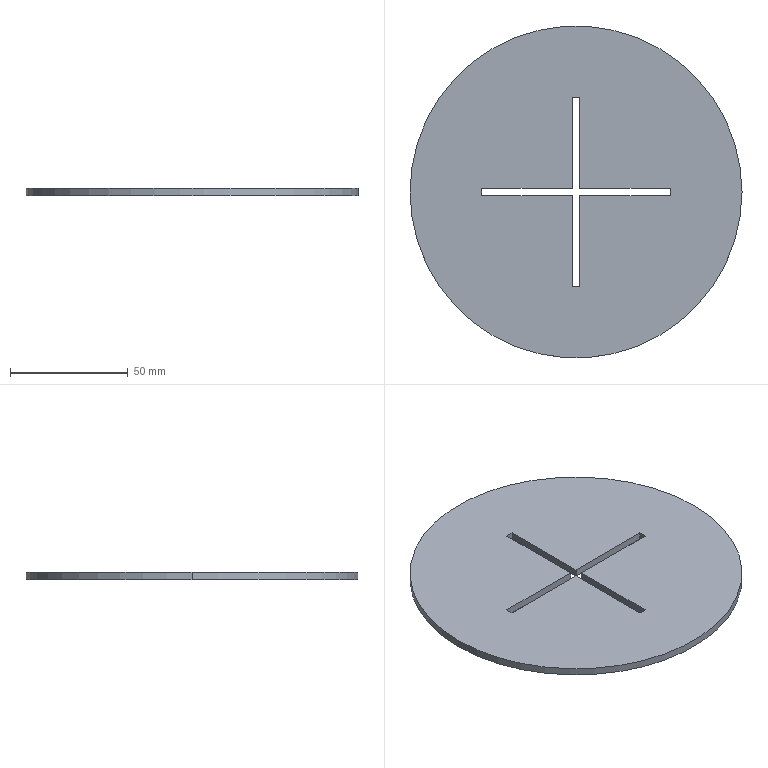Part | SolidWorks | features FlatPattern 1, SMBaseFlange 1, SheetMetal 1 | 1 solid | 16 faces | box 141 x 141 x 3.2 mm | volume 48361 mm3 | plane 14 | cylinder 2 | commonest cylinder face diameters 141 x2
STEP:
#1=CARTESIAN_POINT('',(46.57,-1.6,3.2));
#2=VERTEX_POINT('',#1);
#3=CARTESIAN_POINT('',(-94.43,-1.6,3.2));
#4=VERTEX_POINT('',#3);
#5=CARTESIAN_POINT('',(-23.93,-1.6,3.2));
#6=DIRECTION('',(0.,0.,1.));
#7=DIRECTION('',(1.,0.,0.));
#8=AXIS2_PLACEMENT_3D('',#5,#6,#7);
#9=CIRCLE('',#8,70.5);
#10=EDGE_CURVE('',#2,#4,#9,.T.);
#11=ORIENTED_EDGE('',*,*,#10,.F.);
#12=CARTESIAN_POINT('',(46.57,-1.6,0.));
#13=VERTEX_POINT('',#12);
#14=CARTESIAN_POINT('',(46.57,-1.6,3.2));
#15=DIRECTION('',(0.,0.,-1.));
#16=VECTOR('',#15,1000.);
#17=LINE('',#14,#16);
#18=EDGE_CURVE('',#2,#13,#17,.T.);
#19=ORIENTED_EDGE('',*,*,#18,.T.);
#20=CARTESIAN_POINT('',(-94.43,-1.6,0.));
#21=VERTEX_POINT('',#20);
#22=CARTESIAN_POINT('',(-23.93,-1.6,0.));
#23=DIRECTION('',(0.,0.,1.));
#24=DIRECTION('',(1.,0.,0.));
#25=AXIS2_PLACEMENT_3D('',#22,#23,#24);
#26=CIRCLE('',#25,70.5);
#27=EDGE_CURVE('',#13,#21,#26,.T.);
#28=ORIENTED_EDGE('',*,*,#27,.T.);
#29=CARTESIAN_POINT('',(-94.43,-1.6,3.2));
#30=DIRECTION('',(0.,0.,-1.));
#31=VECTOR('',#30,1000.);
#32=LINE('',#29,#31);
#33=EDGE_CURVE('',#4,#21,#32,.T.);
#34=ORIENTED_EDGE('',*,*,#33,.F.);
#35=EDGE_LOOP('',(#11,#19,#28,#34));
#36=FACE_OUTER_BOUND('',#35,.T.);
#37=CARTESIAN_POINT('',(-23.93,-1.6,3.2));
#38=DIRECTION('',(0.,0.,-1.));
#39=DIRECTION('',(-1.,0.,0.));
#40=AXIS2_PLACEMENT_3D('',#37,#38,#39);
#41=CYLINDRICAL_SURFACE('',#40,70.5);
#42=ADVANCED_FACE('',(#36),#41,.T.);
#43=CARTESIAN_POINT('',(-23.93,-1.6,3.2));
#44=DIRECTION('',(0.,0.,1.));
#45=DIRECTION('',(1.,0.,0.));
#46=AXIS2_PLACEMENT_3D('',#43,#44,#45);
#47=CIRCLE('',#46,70.5);
#48=EDGE_CURVE('',#4,#2,#47,.T.);
#49=ORIENTED_EDGE('',*,*,#48,.T.);
#50=ORIENTED_EDGE('',*,*,#10,.T.);
#51=EDGE_LOOP('',(#49,#50));
#52=FACE_OUTER_BOUND('',#51,.T.);
#53=CARTESIAN_POINT('',(-63.93,-3.2,3.2));
#54=VERTEX_POINT('',#53);
#55=CARTESIAN_POINT('',(-25.53,-3.2,3.2));
#56=VERTEX_POINT('',#55);
#57=CARTESIAN_POINT('',(-63.93,-3.2,3.2));
#58=DIRECTION('',(1.,0.,0.));
#59=VECTOR('',#58,1000.);
#60=LINE('',#57,#59);
#61=EDGE_CURVE('',#54,#56,#60,.T.);
#62=ORIENTED_EDGE('',*,*,#61,.F.);
#63=CARTESIAN_POINT('',(-63.93,0.,3.2));
#64=VERTEX_POINT('',#63);
#65=CARTESIAN_POINT('',(-63.93,0.,3.2));
#66=DIRECTION('',(0.,-1.,0.));
#67=VECTOR('',#66,1000.);
#68=LINE('',#65,#67);
#69=EDGE_CURVE('',#64,#54,#68,.T.);
#70=ORIENTED_EDGE('',*,*,#69,.F.);
#71=CARTESIAN_POINT('',(-25.53,0.,3.2));
#72=VERTEX_POINT('',#71);
#73=CARTESIAN_POINT('',(-25.53,0.,3.2));
#74=DIRECTION('',(-1.,0.,0.));
#75=VECTOR('',#74,1000.);
#76=LINE('',#73,#75);
#77=EDGE_CURVE('',#72,#64,#76,.T.);
#78=ORIENTED_EDGE('',*,*,#77,.F.);
#79=CARTESIAN_POINT('',(-25.53,38.4,3.2));
#80=VERTEX_POINT('',#79);
#81=CARTESIAN_POINT('',(-25.53,38.4,3.2));
#82=DIRECTION('',(0.,-1.,0.));
#83=VECTOR('',#82,1000.);
#84=LINE('',#81,#83);
#85=EDGE_CURVE('',#80,#72,#84,.T.);
#86=ORIENTED_EDGE('',*,*,#85,.F.);
#87=CARTESIAN_POINT('',(-22.33,38.4,3.2));
#88=VERTEX_POINT('',#87);
#89=CARTESIAN_POINT('',(-25.53,38.4,3.2));
#90=DIRECTION('',(-1.,0.,0.));
#91=VECTOR('',#90,1000.);
#92=LINE('',#89,#91);
#93=EDGE_CURVE('',#88,#80,#92,.T.);
#94=ORIENTED_EDGE('',*,*,#93,.F.);
#95=CARTESIAN_POINT('',(-22.33,0.,3.2));
#96=VERTEX_POINT('',#95);
#97=CARTESIAN_POINT('',(-22.33,38.4,3.2));
#98=DIRECTION('',(0.,1.,0.));
#99=VECTOR('',#98,1000.);
#100=LINE('',#97,#99);
#101=EDGE_CURVE('',#96,#88,#100,.T.);
#102=ORIENTED_EDGE('',*,*,#101,.F.);
#103=CARTESIAN_POINT('',(16.07,0.,3.2));
#104=VERTEX_POINT('',#103);
#105=CARTESIAN_POINT('',(16.07,0.,3.2));
#106=DIRECTION('',(-1.,0.,0.));
#107=VECTOR('',#106,1000.);
#108=LINE('',#105,#107);
#109=EDGE_CURVE('',#104,#96,#108,.T.);
#110=ORIENTED_EDGE('',*,*,#109,.F.);
#111=CARTESIAN_POINT('',(16.07,-3.2,3.2));
#112=VERTEX_POINT('',#111);
#113=CARTESIAN_POINT('',(16.07,-3.2,3.2));
#114=DIRECTION('',(0.,1.,0.));
#115=VECTOR('',#114,1000.);
#116=LINE('',#113,#115);
#117=EDGE_CURVE('',#112,#104,#116,.T.);
#118=ORIENTED_EDGE('',*,*,#117,.F.);
#119=CARTESIAN_POINT('',(-22.33,-3.2,3.2));
#120=VERTEX_POINT('',#119);
#121=CARTESIAN_POINT('',(-22.33,-3.2,3.2));
#122=DIRECTION('',(1.,0.,0.));
#123=VECTOR('',#122,1000.);
#124=LINE('',#121,#123);
#125=EDGE_CURVE('',#120,#112,#124,.T.);
#126=ORIENTED_EDGE('',*,*,#125,.F.);
#127=CARTESIAN_POINT('',(-22.33,-41.6,3.2));
#128=VERTEX_POINT('',#127);
#129=CARTESIAN_POINT('',(-22.33,-3.2,3.2));
#130=DIRECTION('',(0.,1.,0.));
#131=VECTOR('',#130,1000.);
#132=LINE('',#129,#131);
#133=EDGE_CURVE('',#128,#120,#132,.T.);
#134=ORIENTED_EDGE('',*,*,#133,.F.);
#135=CARTESIAN_POINT('',(-25.53,-41.6,3.2));
#136=VERTEX_POINT('',#135);
#137=CARTESIAN_POINT('',(-25.53,-41.6,3.2));
#138=DIRECTION('',(1.,0.,0.));
#139=VECTOR('',#138,1000.);
#140=LINE('',#137,#139);
#141=EDGE_CURVE('',#136,#128,#140,.T.);
#142=ORIENTED_EDGE('',*,*,#141,.F.);
#143=CARTESIAN_POINT('',(-25.53,-3.2,3.2));
#144=DIRECTION('',(0.,-1.,0.));
#145=VECTOR('',#144,1000.);
#146=LINE('',#143,#145);
#147=EDGE_CURVE('',#56,#136,#146,.T.);
#148=ORIENTED_EDGE('',*,*,#147,.F.);
#149=EDGE_LOOP('',(#62,#70,#78,#86,#94,#102,#110,#118,#126,#134,#142,#148));
#150=FACE_BOUND('',#149,.T.);
#151=CARTESIAN_POINT('',(-23.93,-1.6,3.2));
#152=DIRECTION('',(0.,0.,1.));
#153=DIRECTION('',(1.,0.,0.));
#154=AXIS2_PLACEMENT_3D('',#151,#152,#153);
#155=PLANE('',#154);
#156=ADVANCED_FACE('',(#52,#150),#155,.T.);
#157=CARTESIAN_POINT('',(-23.93,-1.6,0.));
#158=DIRECTION('',(0.,0.,1.));
#159=DIRECTION('',(1.,0.,0.));
#160=AXIS2_PLACEMENT_3D('',#157,#158,#159);
#161=CIRCLE('',#160,70.5);
#162=EDGE_CURVE('',#21,#13,#161,.T.);
#163=ORIENTED_EDGE('',*,*,#162,.F.);
#164=ORIENTED_EDGE('',*,*,#27,.F.);
#165=EDGE_LOOP('',(#163,#164));
#166=FACE_OUTER_BOUND('',#165,.T.);
#167=CARTESIAN_POINT('',(-63.93,0.,0.));
#168=VERTEX_POINT('',#167);
#169=CARTESIAN_POINT('',(-63.93,-3.2,0.));
#170=VERTEX_POINT('',#169);
#171=CARTESIAN_POINT('',(-63.93,0.,0.));
#172=DIRECTION('',(0.,-1.,0.));
#173=VECTOR('',#172,1000.);
#174=LINE('',#171,#173);
#175=EDGE_CURVE('',#168,#170,#174,.T.);
#176=ORIENTED_EDGE('',*,*,#175,.T.);
#177=CARTESIAN_POINT('',(-25.53,-3.2,0.));
#178=VERTEX_POINT('',#177);
#179=CARTESIAN_POINT('',(-63.93,-3.2,0.));
#180=DIRECTION('',(1.,0.,0.));
#181=VECTOR('',#180,1000.);
#182=LINE('',#179,#181);
#183=EDGE_CURVE('',#170,#178,#182,.T.);
#184=ORIENTED_EDGE('',*,*,#183,.T.);
#185=CARTESIAN_POINT('',(-25.53,-41.6,0.));
#186=VERTEX_POINT('',#185);
#187=CARTESIAN_POINT('',(-25.53,-3.2,0.));
#188=DIRECTION('',(0.,-1.,0.));
#189=VECTOR('',#188,1000.);
#190=LINE('',#187,#189);
#191=EDGE_CURVE('',#178,#186,#190,.T.);
#192=ORIENTED_EDGE('',*,*,#191,.T.);
#193=CARTESIAN_POINT('',(-22.33,-41.6,0.));
#194=VERTEX_POINT('',#193);
#195=CARTESIAN_POINT('',(-25.53,-41.6,0.));
#196=DIRECTION('',(1.,0.,0.));
#197=VECTOR('',#196,1000.);
#198=LINE('',#195,#197);
#199=EDGE_CURVE('',#186,#194,#198,.T.);
#200=ORIENTED_EDGE('',*,*,#199,.T.);
#201=CARTESIAN_POINT('',(-22.33,-3.2,0.));
#202=VERTEX_POINT('',#201);
#203=CARTESIAN_POINT('',(-22.33,-3.2,0.));
#204=DIRECTION('',(0.,1.,0.));
#205=VECTOR('',#204,1000.);
#206=LINE('',#203,#205);
#207=EDGE_CURVE('',#194,#202,#206,.T.);
#208=ORIENTED_EDGE('',*,*,#207,.T.);
#209=CARTESIAN_POINT('',(16.07,-3.2,0.));
#210=VERTEX_POINT('',#209);
#211=CARTESIAN_POINT('',(-22.33,-3.2,0.));
#212=DIRECTION('',(1.,0.,0.));
#213=VECTOR('',#212,1000.);
#214=LINE('',#211,#213);
#215=EDGE_CURVE('',#202,#210,#214,.T.);
#216=ORIENTED_EDGE('',*,*,#215,.T.);
#217=CARTESIAN_POINT('',(16.07,0.,0.));
#218=VERTEX_POINT('',#217);
#219=CARTESIAN_POINT('',(16.07,-3.2,0.));
#220=DIRECTION('',(0.,1.,0.));
#221=VECTOR('',#220,1000.);
#222=LINE('',#219,#221);
#223=EDGE_CURVE('',#210,#218,#222,.T.);
#224=ORIENTED_EDGE('',*,*,#223,.T.);
#225=CARTESIAN_POINT('',(-22.33,0.,0.));
#226=VERTEX_POINT('',#225);
#227=CARTESIAN_POINT('',(16.07,0.,0.));
#228=DIRECTION('',(-1.,0.,0.));
#229=VECTOR('',#228,1000.);
#230=LINE('',#227,#229);
#231=EDGE_CURVE('',#218,#226,#230,.T.);
#232=ORIENTED_EDGE('',*,*,#231,.T.);
#233=CARTESIAN_POINT('',(-22.33,38.4,0.));
#234=VERTEX_POINT('',#233);
#235=CARTESIAN_POINT('',(-22.33,38.4,0.));
#236=DIRECTION('',(0.,1.,0.));
#237=VECTOR('',#236,1000.);
#238=LINE('',#235,#237);
#239=EDGE_CURVE('',#226,#234,#238,.T.);
#240=ORIENTED_EDGE('',*,*,#239,.T.);
#241=CARTESIAN_POINT('',(-25.53,38.4,0.));
#242=VERTEX_POINT('',#241);
#243=CARTESIAN_POINT('',(-25.53,38.4,0.));
#244=DIRECTION('',(-1.,0.,0.));
#245=VECTOR('',#244,1000.);
#246=LINE('',#243,#245);
#247=EDGE_CURVE('',#234,#242,#246,.T.);
#248=ORIENTED_EDGE('',*,*,#247,.T.);
#249=CARTESIAN_POINT('',(-25.53,0.,0.));
#250=VERTEX_POINT('',#249);
#251=CARTESIAN_POINT('',(-25.53,38.4,0.));
#252=DIRECTION('',(0.,-1.,0.));
#253=VECTOR('',#252,1000.);
#254=LINE('',#251,#253);
#255=EDGE_CURVE('',#242,#250,#254,.T.);
#256=ORIENTED_EDGE('',*,*,#255,.T.);
#257=CARTESIAN_POINT('',(-25.53,0.,0.));
#258=DIRECTION('',(-1.,0.,0.));
#259=VECTOR('',#258,1000.);
#260=LINE('',#257,#259);
#261=EDGE_CURVE('',#250,#168,#260,.T.);
#262=ORIENTED_EDGE('',*,*,#261,.T.);
#263=EDGE_LOOP('',(#176,#184,#192,#200,#208,#216,#224,#232,#240,#248,#256,#262));
#264=FACE_BOUND('',#263,.T.);
#265=CARTESIAN_POINT('',(-23.93,-1.6,0.));
#266=DIRECTION('',(0.,0.,1.));
#267=DIRECTION('',(1.,0.,0.));
#268=AXIS2_PLACEMENT_3D('',#265,#266,#267);
#269=PLANE('',#268);
#270=ADVANCED_FACE('',(#166,#264),#269,.F.);
#271=ORIENTED_EDGE('',*,*,#18,.F.);
#272=ORIENTED_EDGE('',*,*,#48,.F.);
#273=ORIENTED_EDGE('',*,*,#33,.T.);
#274=ORIENTED_EDGE('',*,*,#162,.T.);
#275=EDGE_LOOP('',(#271,#272,#273,#274));
#276=FACE_OUTER_BOUND('',#275,.T.);
#277=CARTESIAN_POINT('',(-23.93,-1.6,3.2));
#278=DIRECTION('',(0.,0.,-1.));
#279=DIRECTION('',(-1.,0.,0.));
#280=AXIS2_PLACEMENT_3D('',#277,#278,#279);
#281=CYLINDRICAL_SURFACE('',#280,70.5);
#282=ADVANCED_FACE('',(#276),#281,.T.);
#283=ORIENTED_EDGE('',*,*,#175,.F.);
#284=CARTESIAN_POINT('',(-63.93,0.,3.2));
#285=DIRECTION('',(0.,0.,-1.));
#286=VECTOR('',#285,1000.);
#287=LINE('',#284,#286);
#288=EDGE_CURVE('',#64,#168,#287,.T.);
#289=ORIENTED_EDGE('',*,*,#288,.F.);
#290=ORIENTED_EDGE('',*,*,#69,.T.);
#291=CARTESIAN_POINT('',(-63.93,-3.2,3.2));
#292=DIRECTION('',(0.,0.,-1.));
#293=VECTOR('',#292,1000.);
#294=LINE('',#291,#293);
#295=EDGE_CURVE('',#54,#170,#294,.T.);
#296=ORIENTED_EDGE('',*,*,#295,.T.);
#297=EDGE_LOOP('',(#283,#289,#290,#296));
#298=FACE_OUTER_BOUND('',#297,.T.);
#299=CARTESIAN_POINT('',(-63.93,0.,3.2));
#300=DIRECTION('',(1.,0.,0.));
#301=DIRECTION('',(0.,0.,-1.));
#302=AXIS2_PLACEMENT_3D('',#299,#300,#301);
#303=PLANE('',#302);
#304=ADVANCED_FACE('',(#298),#303,.T.);
#305=ORIENTED_EDGE('',*,*,#183,.F.);
#306=ORIENTED_EDGE('',*,*,#295,.F.);
#307=ORIENTED_EDGE('',*,*,#61,.T.);
#308=CARTESIAN_POINT('',(-25.53,-3.2,3.2));
#309=DIRECTION('',(0.,0.,-1.));
#310=VECTOR('',#309,1000.);
#311=LINE('',#308,#310);
#312=EDGE_CURVE('',#56,#178,#311,.T.);
#313=ORIENTED_EDGE('',*,*,#312,.T.);
#314=EDGE_LOOP('',(#305,#306,#307,#313));
#315=FACE_OUTER_BOUND('',#314,.T.);
#316=CARTESIAN_POINT('',(-63.93,-3.2,3.2));
#317=DIRECTION('',(0.,1.,0.));
#318=DIRECTION('',(-1.,0.,0.));
#319=AXIS2_PLACEMENT_3D('',#316,#317,#318);
#320=PLANE('',#319);
#321=ADVANCED_FACE('',(#315),#320,.T.);
#322=ORIENTED_EDGE('',*,*,#191,.F.);
#323=ORIENTED_EDGE('',*,*,#312,.F.);
#324=ORIENTED_EDGE('',*,*,#147,.T.);
#325=CARTESIAN_POINT('',(-25.53,-41.6,3.2));
#326=DIRECTION('',(0.,0.,-1.));
#327=VECTOR('',#326,1000.);
#328=LINE('',#325,#327);
#329=EDGE_CURVE('',#136,#186,#328,.T.);
#330=ORIENTED_EDGE('',*,*,#329,.T.);
#331=EDGE_LOOP('',(#322,#323,#324,#330));
#332=FACE_OUTER_BOUND('',#331,.T.);
#333=CARTESIAN_POINT('',(-25.53,-3.2,3.2));
#334=DIRECTION('',(1.,0.,0.));
#335=DIRECTION('',(0.,1.,0.));
#336=AXIS2_PLACEMENT_3D('',#333,#334,#335);
#337=PLANE('',#336);
#338=ADVANCED_FACE('',(#332),#337,.T.);
#339=ORIENTED_EDGE('',*,*,#199,.F.);
#340=ORIENTED_EDGE('',*,*,#329,.F.);
#341=ORIENTED_EDGE('',*,*,#141,.T.);
#342=CARTESIAN_POINT('',(-22.33,-41.6,3.2));
#343=DIRECTION('',(0.,0.,-1.));
#344=VECTOR('',#343,1000.);
#345=LINE('',#342,#344);
#346=EDGE_CURVE('',#128,#194,#345,.T.);
#347=ORIENTED_EDGE('',*,*,#346,.T.);
#348=EDGE_LOOP('',(#339,#340,#341,#347));
#349=FACE_OUTER_BOUND('',#348,.T.);
#350=CARTESIAN_POINT('',(-25.53,-41.6,3.2));
#351=DIRECTION('',(0.,1.,0.));
#352=DIRECTION('',(0.,0.,1.));
#353=AXIS2_PLACEMENT_3D('',#350,#351,#352);
#354=PLANE('',#353);
#355=ADVANCED_FACE('',(#349),#354,.T.);
#356=ORIENTED_EDGE('',*,*,#207,.F.);
#357=ORIENTED_EDGE('',*,*,#346,.F.);
#358=ORIENTED_EDGE('',*,*,#133,.T.);
#359=CARTESIAN_POINT('',(-22.33,-3.2,3.2));
#360=DIRECTION('',(0.,0.,-1.));
#361=VECTOR('',#360,1000.);
#362=LINE('',#359,#361);
#363=EDGE_CURVE('',#120,#202,#362,.T.);
#364=ORIENTED_EDGE('',*,*,#363,.T.);
#365=EDGE_LOOP('',(#356,#357,#358,#364));
#366=FACE_OUTER_BOUND('',#365,.T.);
#367=CARTESIAN_POINT('',(-22.33,-3.2,3.2));
#368=DIRECTION('',(-1.,0.,0.));
#369=DIRECTION('',(0.,-1.,0.));
#370=AXIS2_PLACEMENT_3D('',#367,#368,#369);
#371=PLANE('',#370);
#372=ADVANCED_FACE('',(#366),#371,.T.);
#373=ORIENTED_EDGE('',*,*,#215,.F.);
#374=ORIENTED_EDGE('',*,*,#363,.F.);
#375=ORIENTED_EDGE('',*,*,#125,.T.);
#376=CARTESIAN_POINT('',(16.07,-3.2,3.2));
#377=DIRECTION('',(0.,0.,-1.));
#378=VECTOR('',#377,1000.);
#379=LINE('',#376,#378);
#380=EDGE_CURVE('',#112,#210,#379,.T.);
#381=ORIENTED_EDGE('',*,*,#380,.T.);
#382=EDGE_LOOP('',(#373,#374,#375,#381));
#383=FACE_OUTER_BOUND('',#382,.T.);
#384=CARTESIAN_POINT('',(-22.33,-3.2,3.2));
#385=DIRECTION('',(0.,1.,0.));
#386=DIRECTION('',(-1.,0.,0.));
#387=AXIS2_PLACEMENT_3D('',#384,#385,#386);
#388=PLANE('',#387);
#389=ADVANCED_FACE('',(#383),#388,.T.);
#390=ORIENTED_EDGE('',*,*,#223,.F.);
#391=ORIENTED_EDGE('',*,*,#380,.F.);
#392=ORIENTED_EDGE('',*,*,#117,.T.);
#393=CARTESIAN_POINT('',(16.07,0.,3.2));
#394=DIRECTION('',(0.,0.,-1.));
#395=VECTOR('',#394,1000.);
#396=LINE('',#393,#395);
#397=EDGE_CURVE('',#104,#218,#396,.T.);
#398=ORIENTED_EDGE('',*,*,#397,.T.);
#399=EDGE_LOOP('',(#390,#391,#392,#398));
#400=FACE_OUTER_BOUND('',#399,.T.);
#401=CARTESIAN_POINT('',(16.07,-3.2,3.2));
#402=DIRECTION('',(-1.,0.,0.));
#403=DIRECTION('',(0.,0.,1.));
#404=AXIS2_PLACEMENT_3D('',#401,#402,#403);
#405=PLANE('',#404);
#406=ADVANCED_FACE('',(#400),#405,.T.);
#407=ORIENTED_EDGE('',*,*,#231,.F.);
#408=ORIENTED_EDGE('',*,*,#397,.F.);
#409=ORIENTED_EDGE('',*,*,#109,.T.);
#410=CARTESIAN_POINT('',(-22.33,0.,3.2));
#411=DIRECTION('',(0.,0.,-1.));
#412=VECTOR('',#411,1000.);
#413=LINE('',#410,#412);
#414=EDGE_CURVE('',#96,#226,#413,.T.);
#415=ORIENTED_EDGE('',*,*,#414,.T.);
#416=EDGE_LOOP('',(#407,#408,#409,#415));
#417=FACE_OUTER_BOUND('',#416,.T.);
#418=CARTESIAN_POINT('',(16.07,0.,3.2));
#419=DIRECTION('',(0.,-1.,0.));
#420=DIRECTION('',(0.,0.,-1.));
#421=AXIS2_PLACEMENT_3D('',#418,#419,#420);
#422=PLANE('',#421);
#423=ADVANCED_FACE('',(#417),#422,.T.);
#424=ORIENTED_EDGE('',*,*,#239,.F.);
#425=ORIENTED_EDGE('',*,*,#414,.F.);
#426=ORIENTED_EDGE('',*,*,#101,.T.);
#427=CARTESIAN_POINT('',(-22.33,38.4,3.2));
#428=DIRECTION('',(0.,0.,-1.));
#429=VECTOR('',#428,1000.);
#430=LINE('',#427,#429);
#431=EDGE_CURVE('',#88,#234,#430,.T.);
#432=ORIENTED_EDGE('',*,*,#431,.T.);
#433=EDGE_LOOP('',(#424,#425,#426,#432));
#434=FACE_OUTER_BOUND('',#433,.T.);
#435=CARTESIAN_POINT('',(-22.33,38.4,3.2));
#436=DIRECTION('',(-1.,0.,0.));
#437=DIRECTION('',(0.,-1.,0.));
#438=AXIS2_PLACEMENT_3D('',#435,#436,#437);
#439=PLANE('',#438);
#440=ADVANCED_FACE('',(#434),#439,.T.);
#441=ORIENTED_EDGE('',*,*,#247,.F.);
#442=ORIENTED_EDGE('',*,*,#431,.F.);
#443=ORIENTED_EDGE('',*,*,#93,.T.);
#444=CARTESIAN_POINT('',(-25.53,38.4,3.2));
#445=DIRECTION('',(0.,0.,-1.));
#446=VECTOR('',#445,1000.);
#447=LINE('',#444,#446);
#448=EDGE_CURVE('',#80,#242,#447,.T.);
#449=ORIENTED_EDGE('',*,*,#448,.T.);
#450=EDGE_LOOP('',(#441,#442,#443,#449));
#451=FACE_OUTER_BOUND('',#450,.T.);
#452=CARTESIAN_POINT('',(-25.53,38.4,3.2));
#453=DIRECTION('',(0.,-1.,0.));
#454=DIRECTION('',(0.,0.,-1.));
#455=AXIS2_PLACEMENT_3D('',#452,#453,#454);
#456=PLANE('',#455);
#457=ADVANCED_FACE('',(#451),#456,.T.);
#458=ORIENTED_EDGE('',*,*,#255,.F.);
#459=ORIENTED_EDGE('',*,*,#448,.F.);
#460=ORIENTED_EDGE('',*,*,#85,.T.);
#461=CARTESIAN_POINT('',(-25.53,0.,3.2));
#462=DIRECTION('',(0.,0.,-1.));
#463=VECTOR('',#462,1000.);
#464=LINE('',#461,#463);
#465=EDGE_CURVE('',#72,#250,#464,.T.);
#466=ORIENTED_EDGE('',*,*,#465,.T.);
#467=EDGE_LOOP('',(#458,#459,#460,#466));
#468=FACE_OUTER_BOUND('',#467,.T.);
#469=CARTESIAN_POINT('',(-25.53,38.4,3.2));
#470=DIRECTION('',(1.,0.,0.));
#471=DIRECTION('',(0.,1.,0.));
#472=AXIS2_PLACEMENT_3D('',#469,#470,#471);
#473=PLANE('',#472);
#474=ADVANCED_FACE('',(#468),#473,.T.);
#475=ORIENTED_EDGE('',*,*,#261,.F.);
#476=ORIENTED_EDGE('',*,*,#465,.F.);
#477=ORIENTED_EDGE('',*,*,#77,.T.);
#478=ORIENTED_EDGE('',*,*,#288,.T.);
#479=EDGE_LOOP('',(#475,#476,#477,#478));
#480=FACE_OUTER_BOUND('',#479,.T.);
#481=CARTESIAN_POINT('',(-25.53,0.,3.2));
#482=DIRECTION('',(0.,-1.,0.));
#483=DIRECTION('',(0.,0.,-1.));
#484=AXIS2_PLACEMENT_3D('',#481,#482,#483);
#485=PLANE('',#484);
#486=ADVANCED_FACE('',(#480),#485,.T.);
#487=CLOSED_SHELL('',(#42,#156,#270,#282,#304,#321,#338,#355,#372,#389,#406,#423,#440,#457,#474,#486));
#488=MANIFOLD_SOLID_BREP('',#487);
#489=CARTESIAN_POINT('',(0.,0.,0.));
#490=DIRECTION('',(0.,0.,1.));
#491=DIRECTION('',(1.,0.,0.));
#492=AXIS2_PLACEMENT_3D('',#489,#490,#491);
#493=(LENGTH_UNIT()NAMED_UNIT(*)SI_UNIT(.MILLI.,.METRE.));
#494=UNCERTAINTY_MEASURE_WITH_UNIT(LENGTH_MEASURE(0.00001),#493,'','');
#495=(NAMED_UNIT(*)PLANE_ANGLE_UNIT()SI_UNIT($,.RADIAN.));
#496=(NAMED_UNIT(*)SI_UNIT($,.STERADIAN.)SOLID_ANGLE_UNIT());
#497=(GEOMETRIC_REPRESENTATION_CONTEXT(3)GLOBAL_UNCERTAINTY_ASSIGNED_CONTEXT((#494))GLOBAL_UNIT_ASSIGNED_CONTEXT((#493,#495,#496))REPRESENTATION_CONTEXT('',''));
#498=ADVANCED_BREP_SHAPE_REPRESENTATION('',(#488,#492),#497);